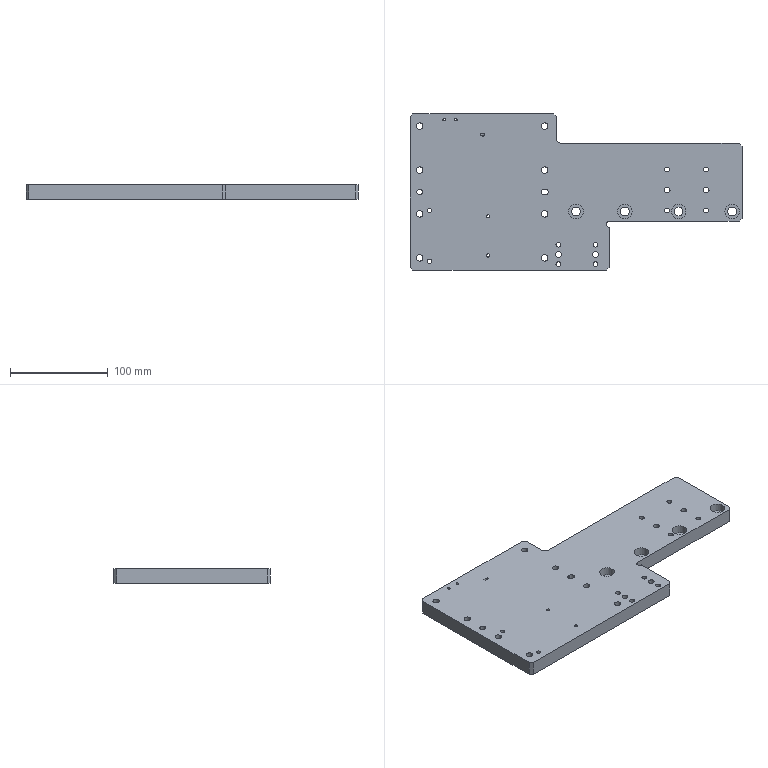Part | 1 solid | 83 faces | box 340 x 160 x 15 mm | volume 606340 mm3 | cylinder 48 | plane 33 | spline 1 | cone 1 | commonest cylinder face diameters 5 x8 6 x8 6.6 x8 11 x8 9 x4 15 x4